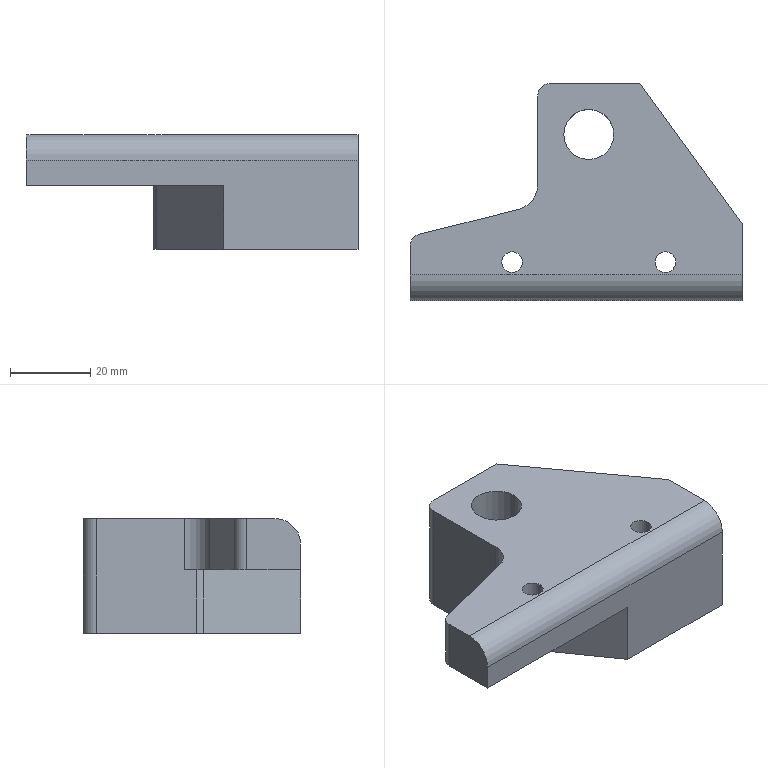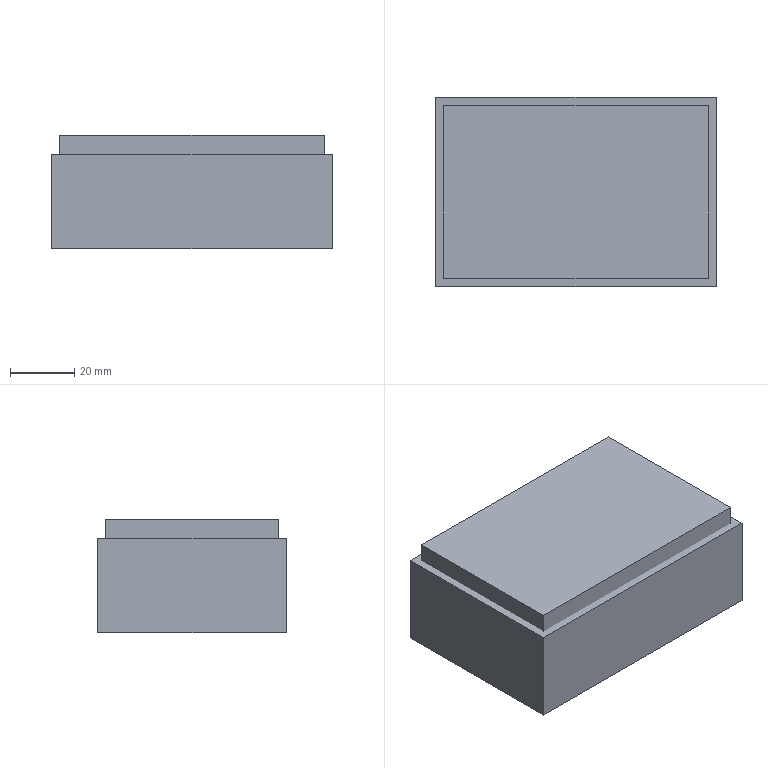CAM job | NX | 3-axis milling, drilling | part box 82.55 x 53.975 x 28.575 mm | stock box 87.55 x 58.975 x 35.575 mm
Tools:
number,name,description,diameter,corner_radius,flute_length,length,flutes
19,D80,Milling Tool-5 Parameters,80.0,0.0,50.0,75.0,2
15,D10JING,Milling Tool-5 Parameters,10.0,0.0,50.0,75.0,2
1,D6A45,Milling Tool-5 Parameters,6.0,0.0,50.0,75.0,2
17,5.2ZT,Drilling Tool,5.1,0.0,35.0,50.0,2
18,4.9ZT,Drilling Tool,4.9,0.0,35.0,50.0,2
16,D6R0.5,Milling Tool-5 Parameters,6.0,0.5,50.0,75.0,2
Operations:
program,operation,operation_type,tool,method,geometry_group,spindle_rpm,surface_speed,feed_per_tooth,feed_cut,feed_plunge,cut_length_mm,path_length_mm,cut_time_min,machine_time_min
1,FLOOR_WALL,VolumeBased25DMillingOperation,D80,METHOD,A,6500.0,1633.0,0.0962,1250.0,100.0,179.55,233.55,0.1436,0.149
1,CAVITY_MILL,CavityMilling,D10JING,METHOD,A,9500.0,298.0,0.1842,3500.0,1000.0,25296.21,26053.747,7.431,7.506
1,CAVITY_MILL_COPY,CavityMilling,D10JING,METHOD,A,9500.0,298.0,0.1842,3500.0,1000.0,3032.276,3327.671,0.9714,1.001
1,FLOOR_WALL_1,VolumeBased25DMillingOperation,D10JING,METHOD,A,9500.0,298.0,0.0658,1250.0,100.0,340.102,525.609,0.2721,0.2906
1,ZLEVEL_PROFILE,ZLevelMilling,D10JING,METHOD,A,9500.0,298.0,0.0658,1250.0,100.0,568.616,773.806,0.4549,0.4754
1,DRILLING,Operation,D6A45,METHOD,A,5000.0,94.0,0.025,250.0,0.0,16.0,205.514,0.064,0.083
1,DRILLING_1,Operation,5.2ZT,METHOD,A,2000.0,32.0,0.05,200.0,0.0,53.339,225.77,0.2667,0.2839
1,DRILLING_1_COPY,Operation,4.9ZT,METHOD,A,2000.0,30.0,0.05,200.0,0.0,17.172,94.344,0.0859,0.0936
1,HOLE_MILLING,CylinderMilling,D10JING,METHOD,A,9500.0,298.0,0.0737,1400.0,100.0,838.865,1180.318,0.5992,0.6333
1,PLANAR_MILL,PlanarMilling,D6A45,METHOD,A,9500.0,179.0,0.0658,1250.0,100.0,292.509,593.999,0.234,0.2642
1,PLANAR_MILL_COPY,PlanarMilling,D6A45,METHOD,A,9500.0,179.0,0.0658,1250.0,100.0,150.853,352.003,0.1207,0.1408
2,FLOOR_WALL_COPY,VolumeBased25DMillingOperation,D80,METHOD,B,6500.0,1633.0,0.0962,1250.0,100.0,1221.85,2569.152,0.9775,1.112
2,ZLEVEL_PROFILE_1,ZLevelMilling,D6R0.5,METHOD,B,9500.0,179.0,0.1842,3500.0,100.0,6086.021,6146.829,1.739,1.745
2,PLANAR_MILL_COPY_1,PlanarMilling,D6A45,METHOD,B,9500.0,179.0,0.0658,1250.0,100.0,325.92,676.225,0.2607,0.2958